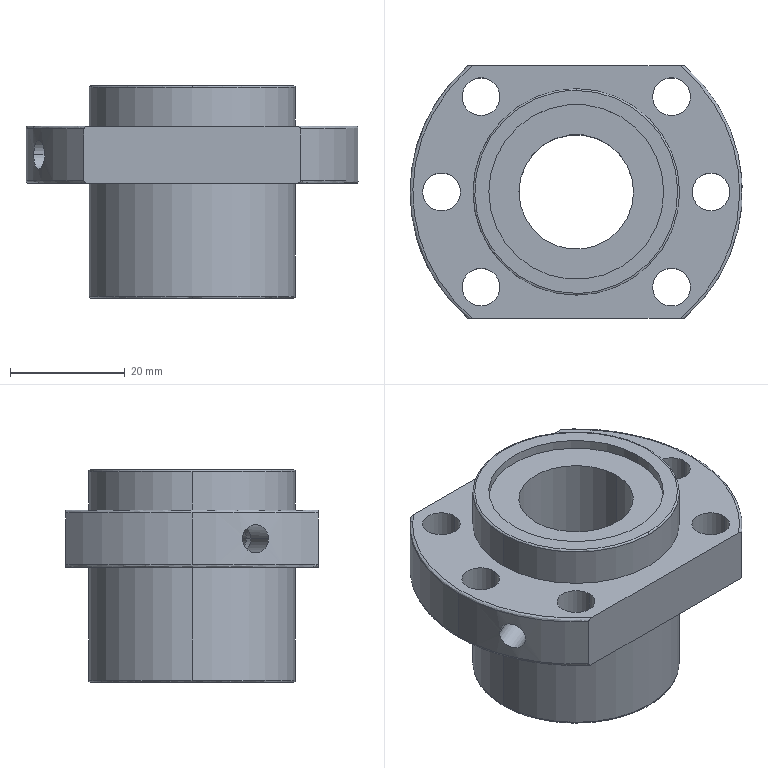Part | SolidWorks | features BaseBody 1 | 1 solid | 47 faces | box 58 x 44 x 37 mm | volume 34920 mm3 | cylinder 29 | spline 8 | plane 8 | cone 2 | commonest cylinder face diameters 6.6 x12 30.5 x4 36 x4 58 x3 4 x2 4.917 x2